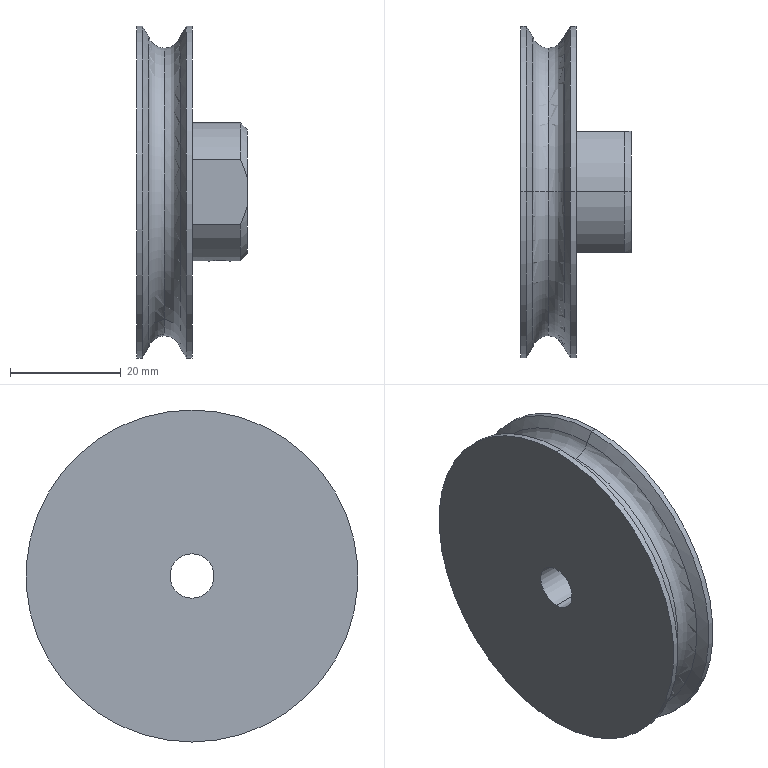Part | STEP file | 11-MBR58_3_P811 | 1 solid | 31 faces | box 20 x 60 x 60 mm | volume 27879 mm3 | cylinder 13 | cone 9 | plane 5 | torus 4 | commonest cylinder face diameters 3.242 x4 60 x4 25 x3 8 x2
STEP:
#1=CARTESIAN_POINT('',(-2.85,0.,28.064));
#2=VERTEX_POINT('',#1);
#3=CARTESIAN_POINT('',(0.,0.,26.));
#4=VERTEX_POINT('',#3);
#5=CARTESIAN_POINT('',(0.,0.,29.));
#6=DIRECTION('',(0.,-1.,0.));
#7=DIRECTION('',(0.,0.,-1.));
#8=AXIS2_PLACEMENT_3D('',#5,#6,#7);
#9=CIRCLE('',#8,3.);
#10=EDGE_CURVE('',#2,#4,#9,.T.);
#11=ORIENTED_EDGE('',*,*,#10,.T.);
#12=CARTESIAN_POINT('',(0.,0.,-26.));
#13=VERTEX_POINT('',#12);
#14=CARTESIAN_POINT('',(0.,0.,0.));
#15=DIRECTION('',(-1.,0.,0.));
#16=DIRECTION('',(0.,0.,1.));
#17=AXIS2_PLACEMENT_3D('',#14,#15,#16);
#18=CIRCLE('',#17,26.);
#19=EDGE_CURVE('',#4,#13,#18,.T.);
#20=ORIENTED_EDGE('',*,*,#19,.T.);
#21=CARTESIAN_POINT('',(-2.85,0.,-28.064));
#22=VERTEX_POINT('',#21);
#23=CARTESIAN_POINT('',(0.,0.,-29.));
#24=DIRECTION('',(0.,1.,0.));
#25=DIRECTION('',(0.,0.,1.));
#26=AXIS2_PLACEMENT_3D('',#23,#24,#25);
#27=CIRCLE('',#26,3.);
#28=EDGE_CURVE('',#22,#13,#27,.T.);
#29=ORIENTED_EDGE('',*,*,#28,.F.);
#30=CARTESIAN_POINT('',(-2.85,0.,0.));
#31=DIRECTION('',(-1.,0.,0.));
#32=DIRECTION('',(0.,0.,1.));
#33=AXIS2_PLACEMENT_3D('',#30,#31,#32);
#34=CIRCLE('',#33,28.064);
#35=EDGE_CURVE('',#2,#22,#34,.T.);
#36=ORIENTED_EDGE('',*,*,#35,.F.);
#37=EDGE_LOOP('',(#11,#20,#29,#36));
#38=FACE_OUTER_BOUND('',#37,.T.);
#39=CARTESIAN_POINT('',(0.,0.,0.));
#40=DIRECTION('',(-1.,0.,0.));
#41=DIRECTION('',(0.,0.,1.));
#42=AXIS2_PLACEMENT_3D('',#39,#40,#41);
#43=TOROIDAL_SURFACE('',#42,29.,3.);
#44=ADVANCED_FACE('',(#38),#43,.F.);
#45=ORIENTED_EDGE('',*,*,#28,.T.);
#46=CARTESIAN_POINT('',(0.,0.,0.));
#47=DIRECTION('',(-1.,0.,0.));
#48=DIRECTION('',(0.,0.,1.));
#49=AXIS2_PLACEMENT_3D('',#46,#47,#48);
#50=CIRCLE('',#49,26.);
#51=EDGE_CURVE('',#13,#4,#50,.T.);
#52=ORIENTED_EDGE('',*,*,#51,.T.);
#53=ORIENTED_EDGE('',*,*,#10,.F.);
#54=CARTESIAN_POINT('',(-2.85,0.,0.));
#55=DIRECTION('',(-1.,0.,0.));
#56=DIRECTION('',(0.,0.,1.));
#57=AXIS2_PLACEMENT_3D('',#54,#55,#56);
#58=CIRCLE('',#57,28.064);
#59=EDGE_CURVE('',#22,#2,#58,.T.);
#60=ORIENTED_EDGE('',*,*,#59,.F.);
#61=EDGE_LOOP('',(#45,#52,#53,#60));
#62=FACE_OUTER_BOUND('',#61,.T.);
#63=CARTESIAN_POINT('',(0.,0.,0.));
#64=DIRECTION('',(-1.,0.,0.));
#65=DIRECTION('',(0.,0.,1.));
#66=AXIS2_PLACEMENT_3D('',#63,#64,#65);
#67=TOROIDAL_SURFACE('',#66,29.,3.);
#68=ADVANCED_FACE('',(#62),#67,.F.);
#69=CARTESIAN_POINT('',(8.379,0.,-4.));
#70=VERTEX_POINT('',#69);
#71=CARTESIAN_POINT('',(11.621,0.,-4.));
#72=VERTEX_POINT('',#71);
#73=CARTESIAN_POINT('',(8.379,0.,-4.));
#74=CARTESIAN_POINT('',(8.379,-0.1084,-4.));
#75=CARTESIAN_POINT('',(8.39,-0.2147,-3.996));
#76=CARTESIAN_POINT('',(8.432,-0.4235,-3.979));
#77=CARTESIAN_POINT('',(8.463,-0.5271,-3.966));
#78=CARTESIAN_POINT('',(8.586,-0.821,-3.92));
#79=CARTESIAN_POINT('',(8.707,-0.9992,-3.876));
#80=CARTESIAN_POINT('',(9.002,-1.295,-3.788));
#81=CARTESIAN_POINT('',(9.181,-1.415,-3.742));
#82=CARTESIAN_POINT('',(9.473,-1.537,-3.693));
#83=CARTESIAN_POINT('',(9.576,-1.568,-3.68));
#84=CARTESIAN_POINT('',(9.786,-1.61,-3.662));
#85=CARTESIAN_POINT('',(9.892,-1.621,-3.657));
#86=CARTESIAN_POINT('',(10.106,-1.621,-3.657));
#87=CARTESIAN_POINT('',(10.215,-1.61,-3.662));
#88=CARTESIAN_POINT('',(10.424,-1.568,-3.68));
#89=CARTESIAN_POINT('',(10.526,-1.537,-3.693));
#90=CARTESIAN_POINT('',(10.723,-1.455,-3.726));
#91=CARTESIAN_POINT('',(10.816,-1.405,-3.746));
#92=CARTESIAN_POINT('',(10.99,-1.288,-3.788));
#93=CARTESIAN_POINT('',(11.073,-1.22,-3.81));
#94=CARTESIAN_POINT('',(11.221,-1.072,-3.855));
#95=CARTESIAN_POINT('',(11.287,-0.9909,-3.876));
#96=CARTESIAN_POINT('',(11.405,-0.8157,-3.917));
#97=CARTESIAN_POINT('',(11.456,-0.7213,-3.936));
#98=CARTESIAN_POINT('',(11.577,-0.429,-3.982));
#99=CARTESIAN_POINT('',(11.621,-0.2135,-4.));
#100=CARTESIAN_POINT('',(11.621,0.,-4.));
#101=B_SPLINE_CURVE_WITH_KNOTS('',3,(#73,#74,#75,#76,#77,#78,#79,#80,#81,#82,#83,#84,#85,#86,#87,#88,#89,#90,#91,#92,#93,#94,#95,#96,#97,#98,#99,#100),.UNSPECIFIED.,.F.,.F.,(4,2,2,2,2,2,2,2,2,2,2,2,2,4),(0.,0.0003202,0.0006405,0.001281,0.001921,0.002242,0.002562,0.002882,0.003202,0.003523,0.003843,0.004163,0.004483,0.005124),.UNSPECIFIED.);
#102=EDGE_CURVE('',#70,#72,#101,.T.);
#103=ORIENTED_EDGE('',*,*,#102,.T.);
#104=CARTESIAN_POINT('',(11.621,0.,-12.121));
#105=VERTEX_POINT('',#104);
#106=CARTESIAN_POINT('',(11.621,0.,-3.));
#107=DIRECTION('',(0.,0.,-1.));
#108=VECTOR('',#107,1000.);
#109=LINE('',#106,#108);
#110=EDGE_CURVE('',#72,#105,#109,.T.);
#111=ORIENTED_EDGE('',*,*,#110,.T.);
#112=CARTESIAN_POINT('',(8.379,0.,-12.121));
#113=VERTEX_POINT('',#112);
#114=CARTESIAN_POINT('',(10.,0.,-12.121));
#115=DIRECTION('',(0.,0.,-1.));
#116=DIRECTION('',(-1.,0.,0.));
#117=AXIS2_PLACEMENT_3D('',#114,#115,#116);
#118=CIRCLE('',#117,1.621);
#119=EDGE_CURVE('',#105,#113,#118,.T.);
#120=ORIENTED_EDGE('',*,*,#119,.T.);
#121=CARTESIAN_POINT('',(8.379,0.,-3.));
#122=DIRECTION('',(0.,0.,-1.));
#123=VECTOR('',#122,1000.);
#124=LINE('',#121,#123);
#125=EDGE_CURVE('',#70,#113,#124,.T.);
#126=ORIENTED_EDGE('',*,*,#125,.F.);
#127=EDGE_LOOP('',(#103,#111,#120,#126));
#128=FACE_OUTER_BOUND('',#127,.T.);
#129=CARTESIAN_POINT('',(10.,0.,-3.));
#130=DIRECTION('',(0.,0.,-1.));
#131=DIRECTION('',(-1.,0.,0.));
#132=AXIS2_PLACEMENT_3D('',#129,#130,#131);
#133=CYLINDRICAL_SURFACE('',#132,1.621);
#134=ADVANCED_FACE('',(#128),#133,.F.);
#135=ORIENTED_EDGE('',*,*,#119,.F.);
#136=CARTESIAN_POINT('',(12.,0.,-12.5));
#137=VERTEX_POINT('',#136);
#138=CARTESIAN_POINT('',(11.621,0.,-12.121));
#139=DIRECTION('',(0.7071,0.,-0.7071));
#140=VECTOR('',#139,1000.);
#141=LINE('',#138,#140);
#142=EDGE_CURVE('',#105,#137,#141,.T.);
#143=ORIENTED_EDGE('',*,*,#142,.T.);
#144=CARTESIAN_POINT('',(8.,0.,-12.5));
#145=VERTEX_POINT('',#144);
#146=CARTESIAN_POINT('',(12.,0.,-12.5));
#147=CARTESIAN_POINT('',(12.,-0.2539,-12.5));
#148=CARTESIAN_POINT('',(11.943,-0.5065,-12.492));
#149=CARTESIAN_POINT('',(11.783,-0.8509,-12.472));
#150=CARTESIAN_POINT('',(11.718,-0.9588,-12.464));
#151=CARTESIAN_POINT('',(11.567,-1.162,-12.446));
#152=CARTESIAN_POINT('',(11.48,-1.256,-12.437));
#153=CARTESIAN_POINT('',(11.199,-1.507,-12.41));
#154=CARTESIAN_POINT('',(10.978,-1.64,-12.392));
#155=CARTESIAN_POINT('',(10.624,-1.772,-12.374));
#156=CARTESIAN_POINT('',(10.5,-1.805,-12.369));
#157=CARTESIAN_POINT('',(10.251,-1.85,-12.362));
#158=CARTESIAN_POINT('',(10.126,-1.861,-12.361));
#159=CARTESIAN_POINT('',(9.873,-1.861,-12.361));
#160=CARTESIAN_POINT('',(9.745,-1.849,-12.362));
#161=CARTESIAN_POINT('',(9.497,-1.805,-12.369));
#162=CARTESIAN_POINT('',(9.376,-1.771,-12.374));
#163=CARTESIAN_POINT('',(9.139,-1.683,-12.386));
#164=CARTESIAN_POINT('',(9.024,-1.628,-12.394));
#165=CARTESIAN_POINT('',(8.808,-1.498,-12.41));
#166=CARTESIAN_POINT('',(8.706,-1.423,-12.419));
#167=CARTESIAN_POINT('',(8.517,-1.253,-12.437));
#168=CARTESIAN_POINT('',(8.432,-1.16,-12.446));
#169=CARTESIAN_POINT('',(8.281,-0.9576,-12.464));
#170=CARTESIAN_POINT('',(8.215,-0.8474,-12.472));
#171=CARTESIAN_POINT('',(8.057,-0.5052,-12.492));
#172=CARTESIAN_POINT('',(8.,-0.2516,-12.5));
#173=CARTESIAN_POINT('',(8.,0.,-12.5));
#174=B_SPLINE_CURVE_WITH_KNOTS('',3,(#146,#147,#148,#149,#150,#151,#152,#153,#154,#155,#156,#157,#158,#159,#160,#161,#162,#163,#164,#165,#166,#167,#168,#169,#170,#171,#172,#173),.UNSPECIFIED.,.F.,.F.,(4,2,2,2,2,2,2,2,2,2,2,2,2,4),(0.007606,0.008363,0.008741,0.00912,0.009877,0.01026,0.01063,0.01101,0.01139,0.01177,0.01215,0.01253,0.0129,0.01366),.UNSPECIFIED.);
#175=EDGE_CURVE('',#137,#145,#174,.T.);
#176=ORIENTED_EDGE('',*,*,#175,.T.);
#177=CARTESIAN_POINT('',(8.379,0.,-12.121));
#178=DIRECTION('',(-0.7071,0.,-0.7071));
#179=VECTOR('',#178,1000.);
#180=LINE('',#177,#179);
#181=EDGE_CURVE('',#113,#145,#180,.T.);
#182=ORIENTED_EDGE('',*,*,#181,.F.);
#183=EDGE_LOOP('',(#135,#143,#176,#182));
#184=FACE_OUTER_BOUND('',#183,.T.);
#185=CARTESIAN_POINT('',(10.,0.,-12.121));
#186=DIRECTION('',(0.,0.,-1.));
#187=DIRECTION('',(-1.,0.,0.));
#188=AXIS2_PLACEMENT_3D('',#185,#186,#187);
#189=CONICAL_SURFACE('',#188,1.621,0.7854);
#190=ADVANCED_FACE('',(#184),#189,.F.);
#191=CARTESIAN_POINT('',(10.,3.657,1.621));
#192=VERTEX_POINT('',#191);
#193=CARTESIAN_POINT('',(10.,3.657,-1.621));
#194=VERTEX_POINT('',#193);
#195=CARTESIAN_POINT('',(10.,3.657,1.621));
#196=CARTESIAN_POINT('',(9.892,3.657,1.621));
#197=CARTESIAN_POINT('',(9.785,3.662,1.61));
#198=CARTESIAN_POINT('',(9.577,3.68,1.568));
#199=CARTESIAN_POINT('',(9.473,3.693,1.537));
#200=CARTESIAN_POINT('',(9.18,3.743,1.414));
#201=CARTESIAN_POINT('',(9.002,3.788,1.294));
#202=CARTESIAN_POINT('',(8.706,3.876,0.9983));
#203=CARTESIAN_POINT('',(8.586,3.92,0.8195));
#204=CARTESIAN_POINT('',(8.464,3.966,0.5273));
#205=CARTESIAN_POINT('',(8.432,3.979,0.4239));
#206=CARTESIAN_POINT('',(8.39,3.996,0.214));
#207=CARTESIAN_POINT('',(8.379,4.,0.108));
#208=CARTESIAN_POINT('',(8.379,4.,-0.1063));
#209=CARTESIAN_POINT('',(8.39,3.996,-0.2149));
#210=CARTESIAN_POINT('',(8.432,3.979,-0.424));
#211=CARTESIAN_POINT('',(8.463,3.967,-0.5259));
#212=CARTESIAN_POINT('',(8.545,3.935,-0.7235));
#213=CARTESIAN_POINT('',(8.596,3.917,-0.8164));
#214=CARTESIAN_POINT('',(8.713,3.876,-0.9909));
#215=CARTESIAN_POINT('',(8.781,3.854,-1.073));
#216=CARTESIAN_POINT('',(8.929,3.81,-1.221));
#217=CARTESIAN_POINT('',(9.01,3.788,-1.288));
#218=CARTESIAN_POINT('',(9.185,3.746,-1.405));
#219=CARTESIAN_POINT('',(9.279,3.726,-1.456));
#220=CARTESIAN_POINT('',(9.571,3.677,-1.577));
#221=CARTESIAN_POINT('',(9.787,3.657,-1.621));
#222=CARTESIAN_POINT('',(10.,3.657,-1.621));
#223=B_SPLINE_CURVE_WITH_KNOTS('',3,(#195,#196,#197,#198,#199,#200,#201,#202,#203,#204,#205,#206,#207,#208,#209,#210,#211,#212,#213,#214,#215,#216,#217,#218,#219,#220,#221,#222),.UNSPECIFIED.,.F.,.F.,(4,2,2,2,2,2,2,2,2,2,2,2,2,4),(0.,0.0003202,0.0006404,0.001281,0.001921,0.002242,0.002562,0.002882,0.003202,0.003522,0.003843,0.004163,0.004483,0.005123),.UNSPECIFIED.);
#224=EDGE_CURVE('',#192,#194,#223,.T.);
#225=ORIENTED_EDGE('',*,*,#224,.T.);
#226=CARTESIAN_POINT('',(10.,11.,-1.621));
#227=VERTEX_POINT('',#226);
#228=CARTESIAN_POINT('',(10.,3.,-1.621));
#229=DIRECTION('',(0.,1.,0.));
#230=VECTOR('',#229,1000.);
#231=LINE('',#228,#230);
#232=EDGE_CURVE('',#194,#227,#231,.T.);
#233=ORIENTED_EDGE('',*,*,#232,.T.);
#234=CARTESIAN_POINT('',(10.,11.,1.621));
#235=VERTEX_POINT('',#234);
#236=CARTESIAN_POINT('',(10.,11.,0.));
#237=DIRECTION('',(0.,-1.,0.));
#238=DIRECTION('',(0.,0.,-1.));
#239=AXIS2_PLACEMENT_3D('',#236,#237,#238);
#240=CIRCLE('',#239,1.621);
#241=EDGE_CURVE('',#235,#227,#240,.T.);
#242=ORIENTED_EDGE('',*,*,#241,.F.);
#243=CARTESIAN_POINT('',(10.,3.,1.621));
#244=DIRECTION('',(0.,1.,0.));
#245=VECTOR('',#244,1000.);
#246=LINE('',#243,#245);
#247=EDGE_CURVE('',#192,#235,#246,.T.);
#248=ORIENTED_EDGE('',*,*,#247,.F.);
#249=EDGE_LOOP('',(#225,#233,#242,#248));
#250=FACE_OUTER_BOUND('',#249,.T.);
#251=CARTESIAN_POINT('',(10.,3.,0.));
#252=DIRECTION('',(0.,1.,0.));
#253=DIRECTION('',(0.,0.,1.));
#254=AXIS2_PLACEMENT_3D('',#251,#252,#253);
#255=CYLINDRICAL_SURFACE('',#254,1.621);
#256=ADVANCED_FACE('',(#250),#255,.F.);
#257=CARTESIAN_POINT('',(5.,0.,30.));
#258=VERTEX_POINT('',#257);
#259=CARTESIAN_POINT('',(5.,0.,-30.));
#260=VERTEX_POINT('',#259);
#261=CARTESIAN_POINT('',(5.,0.,0.));
#262=DIRECTION('',(-1.,0.,0.));
#263=DIRECTION('',(0.,0.,1.));
#264=AXIS2_PLACEMENT_3D('',#261,#262,#263);
#265=CIRCLE('',#264,30.);
#266=EDGE_CURVE('',#258,#260,#265,.T.);
#267=ORIENTED_EDGE('',*,*,#266,.T.);
#268=CARTESIAN_POINT('',(3.968,0.,-30.));
#269=VERTEX_POINT('',#268);
#270=CARTESIAN_POINT('',(15.,0.,-30.));
#271=DIRECTION('',(-1.,0.,0.));
#272=VECTOR('',#271,1000.);
#273=LINE('',#270,#272);
#274=EDGE_CURVE('',#260,#269,#273,.T.);
#275=ORIENTED_EDGE('',*,*,#274,.T.);
#276=CARTESIAN_POINT('',(3.968,0.,30.));
#277=VERTEX_POINT('',#276);
#278=CARTESIAN_POINT('',(3.968,0.,0.));
#279=DIRECTION('',(-1.,0.,0.));
#280=DIRECTION('',(0.,0.,1.));
#281=AXIS2_PLACEMENT_3D('',#278,#279,#280);
#282=CIRCLE('',#281,30.);
#283=EDGE_CURVE('',#277,#269,#282,.T.);
#284=ORIENTED_EDGE('',*,*,#283,.F.);
#285=CARTESIAN_POINT('',(15.,0.,30.));
#286=DIRECTION('',(-1.,0.,0.));
#287=VECTOR('',#286,1000.);
#288=LINE('',#285,#287);
#289=EDGE_CURVE('',#258,#277,#288,.T.);
#290=ORIENTED_EDGE('',*,*,#289,.F.);
#291=EDGE_LOOP('',(#267,#275,#284,#290));
#292=FACE_OUTER_BOUND('',#291,.T.);
#293=CARTESIAN_POINT('',(15.,0.,0.));
#294=DIRECTION('',(-1.,0.,0.));
#295=DIRECTION('',(0.,0.,1.));
#296=AXIS2_PLACEMENT_3D('',#293,#294,#295);
#297=CYLINDRICAL_SURFACE('',#296,30.);
#298=ADVANCED_FACE('',(#292),#297,.T.);
#299=CARTESIAN_POINT('',(2.85,0.,28.064));
#300=VERTEX_POINT('',#299);
#301=CARTESIAN_POINT('',(2.85,0.,-28.064));
#302=VERTEX_POINT('',#301);
#303=CARTESIAN_POINT('',(2.85,0.,0.));
#304=DIRECTION('',(-1.,0.,0.));
#305=DIRECTION('',(0.,0.,1.));
#306=AXIS2_PLACEMENT_3D('',#303,#304,#305);
#307=CIRCLE('',#306,28.064);
#308=EDGE_CURVE('',#300,#302,#307,.T.);
#309=ORIENTED_EDGE('',*,*,#308,.F.);
#310=CARTESIAN_POINT('',(3.968,0.,30.));
#311=DIRECTION('',(0.5,0.,0.866));
#312=VECTOR('',#311,1000.);
#313=LINE('',#310,#312);
#314=EDGE_CURVE('',#300,#277,#313,.T.);
#315=ORIENTED_EDGE('',*,*,#314,.T.);
#316=ORIENTED_EDGE('',*,*,#283,.T.);
#317=CARTESIAN_POINT('',(3.968,0.,-30.));
#318=DIRECTION('',(0.5,0.,-0.866));
#319=VECTOR('',#318,1000.);
#320=LINE('',#317,#319);
#321=EDGE_CURVE('',#302,#269,#320,.T.);
#322=ORIENTED_EDGE('',*,*,#321,.F.);
#323=EDGE_LOOP('',(#309,#315,#316,#322));
#324=FACE_OUTER_BOUND('',#323,.T.);
#325=CARTESIAN_POINT('',(3.968,0.,0.));
#326=DIRECTION('',(1.,0.,0.));
#327=DIRECTION('',(0.,0.,-1.));
#328=AXIS2_PLACEMENT_3D('',#325,#326,#327);
#329=CONICAL_SURFACE('',#328,30.,1.047);
#330=ADVANCED_FACE('',(#324),#329,.T.);
#331=ORIENTED_EDGE('',*,*,#51,.F.);
#332=CARTESIAN_POINT('',(0.,0.,-29.));
#333=DIRECTION('',(0.,1.,0.));
#334=DIRECTION('',(0.,0.,1.));
#335=AXIS2_PLACEMENT_3D('',#332,#333,#334);
#336=CIRCLE('',#335,3.);
#337=EDGE_CURVE('',#13,#302,#336,.T.);
#338=ORIENTED_EDGE('',*,*,#337,.T.);
#339=CARTESIAN_POINT('',(2.85,0.,0.));
#340=DIRECTION('',(-1.,0.,0.));
#341=DIRECTION('',(0.,0.,1.));
#342=AXIS2_PLACEMENT_3D('',#339,#340,#341);
#343=CIRCLE('',#342,28.064);
#344=EDGE_CURVE('',#302,#300,#343,.T.);
#345=ORIENTED_EDGE('',*,*,#344,.T.);
#346=CARTESIAN_POINT('',(0.,0.,29.));
#347=DIRECTION('',(0.,-1.,0.));
#348=DIRECTION('',(0.,0.,-1.));
#349=AXIS2_PLACEMENT_3D('',#346,#347,#348);
#350=CIRCLE('',#349,3.);
#351=EDGE_CURVE('',#4,#300,#350,.T.);
#352=ORIENTED_EDGE('',*,*,#351,.F.);
#353=EDGE_LOOP('',(#331,#338,#345,#352));
#354=FACE_OUTER_BOUND('',#353,.T.);
#355=CARTESIAN_POINT('',(0.,0.,0.));
#356=DIRECTION('',(-1.,0.,0.));
#357=DIRECTION('',(0.,0.,1.));
#358=AXIS2_PLACEMENT_3D('',#355,#356,#357);
#359=TOROIDAL_SURFACE('',#358,29.,3.);
#360=ADVANCED_FACE('',(#354),#359,.F.);
#361=ORIENTED_EDGE('',*,*,#35,.T.);
#362=CARTESIAN_POINT('',(-3.968,0.,-30.));
#363=VERTEX_POINT('',#362);
#364=CARTESIAN_POINT('',(-2.85,0.,-28.064));
#365=DIRECTION('',(-0.5,0.,-0.866));
#366=VECTOR('',#365,1000.);
#367=LINE('',#364,#366);
#368=EDGE_CURVE('',#22,#363,#367,.T.);
#369=ORIENTED_EDGE('',*,*,#368,.T.);
#370=CARTESIAN_POINT('',(-3.968,0.,30.));
#371=VERTEX_POINT('',#370);
#372=CARTESIAN_POINT('',(-3.968,0.,0.));
#373=DIRECTION('',(-1.,0.,0.));
#374=DIRECTION('',(0.,0.,1.));
#375=AXIS2_PLACEMENT_3D('',#372,#373,#374);
#376=CIRCLE('',#375,30.);
#377=EDGE_CURVE('',#371,#363,#376,.T.);
#378=ORIENTED_EDGE('',*,*,#377,.F.);
#379=CARTESIAN_POINT('',(-2.85,0.,28.064));
#380=DIRECTION('',(-0.5,0.,0.866));
#381=VECTOR('',#380,1000.);
#382=LINE('',#379,#381);
#383=EDGE_CURVE('',#2,#371,#382,.T.);
#384=ORIENTED_EDGE('',*,*,#383,.F.);
#385=EDGE_LOOP('',(#361,#369,#378,#384));
#386=FACE_OUTER_BOUND('',#385,.T.);
#387=CARTESIAN_POINT('',(-2.85,0.,0.));
#388=DIRECTION('',(-1.,0.,0.));
#389=DIRECTION('',(0.,0.,1.));
#390=AXIS2_PLACEMENT_3D('',#387,#388,#389);
#391=CONICAL_SURFACE('',#390,28.064,1.047);
#392=ADVANCED_FACE('',(#386),#391,.T.);
#393=ORIENTED_EDGE('',*,*,#377,.T.);
#394=CARTESIAN_POINT('',(-5.,0.,-30.));
#395=VERTEX_POINT('',#394);
#396=CARTESIAN_POINT('',(15.,0.,-30.));
#397=DIRECTION('',(-1.,0.,0.));
#398=VECTOR('',#397,1000.);
#399=LINE('',#396,#398);
#400=EDGE_CURVE('',#363,#395,#399,.T.);
#401=ORIENTED_EDGE('',*,*,#400,.T.);
#402=CARTESIAN_POINT('',(-5.,0.,30.));
#403=VERTEX_POINT('',#402);
#404=CARTESIAN_POINT('',(-5.,0.,0.));
#405=DIRECTION('',(-1.,0.,0.));
#406=DIRECTION('',(0.,0.,1.));
#407=AXIS2_PLACEMENT_3D('',#404,#405,#406);
#408=CIRCLE('',#407,30.);
#409=EDGE_CURVE('',#403,#395,#408,.T.);
#410=ORIENTED_EDGE('',*,*,#409,.F.);
#411=CARTESIAN_POINT('',(15.,0.,30.));
#412=DIRECTION('',(-1.,0.,0.));
#413=VECTOR('',#412,1000.);
#414=LINE('',#411,#413);
#415=EDGE_CURVE('',#371,#403,#414,.T.);
#416=ORIENTED_EDGE('',*,*,#415,.F.);
#417=EDGE_LOOP('',(#393,#401,#410,#416));
#418=FACE_OUTER_BOUND('',#417,.T.);
#419=CARTESIAN_POINT('',(15.,0.,0.));
#420=DIRECTION('',(-1.,0.,0.));
#421=DIRECTION('',(0.,0.,1.));
#422=AXIS2_PLACEMENT_3D('',#419,#420,#421);
#423=CYLINDRICAL_SURFACE('',#422,30.);
#424=ADVANCED_FACE('',(#418),#423,.T.);
#425=CARTESIAN_POINT('',(15.,0.,-4.));
#426=VERTEX_POINT('',#425);
#427=CARTESIAN_POINT('',(15.,0.,4.));
#428=VERTEX_POINT('',#427);
#429=CARTESIAN_POINT('',(15.,0.,0.));
#430=DIRECTION('',(-1.,0.,0.));
#431=DIRECTION('',(0.,0.,1.));
#432=AXIS2_PLACEMENT_3D('',#429,#430,#431);
#433=CIRCLE('',#432,4.);
#434=EDGE_CURVE('',#426,#428,#433,.T.);
#435=ORIENTED_EDGE('',*,*,#434,.F.);
#436=CARTESIAN_POINT('',(15.,0.,-4.));
#437=DIRECTION('',(-1.,0.,0.));
#438=VECTOR('',#437,1000.);
#439=LINE('',#436,#438);
#440=EDGE_CURVE('',#426,#72,#439,.T.);
#441=ORIENTED_EDGE('',*,*,#440,.T.);
#442=ORIENTED_EDGE('',*,*,#102,.F.);
#443=CARTESIAN_POINT('',(-5.,0.,-4.));
#444=VERTEX_POINT('',#443);
#445=CARTESIAN_POINT('',(15.,0.,-4.));
#446=DIRECTION('',(-1.,0.,0.));
#447=VECTOR('',#446,1000.);
#448=LINE('',#445,#447);
#449=EDGE_CURVE('',#70,#444,#448,.T.);
#450=ORIENTED_EDGE('',*,*,#449,.T.);
#451=CARTESIAN_POINT('',(-5.,0.,4.));
#452=VERTEX_POINT('',#451);
#453=CARTESIAN_POINT('',(-5.,0.,0.));
#454=DIRECTION('',(-1.,0.,0.));
#455=DIRECTION('',(0.,0.,1.));
#456=AXIS2_PLACEMENT_3D('',#453,#454,#455);
#457=CIRCLE('',#456,4.);
#458=EDGE_CURVE('',#444,#452,#457,.T.);
#459=ORIENTED_EDGE('',*,*,#458,.T.);
#460=CARTESIAN_POINT('',(15.,0.,4.));
#461=DIRECTION('',(-1.,0.,0.));
#462=VECTOR('',#461,1000.);
#463=LINE('',#460,#462);
#464=EDGE_CURVE('',#428,#452,#463,.T.);
#465=ORIENTED_EDGE('',*,*,#464,.F.);
#466=EDGE_LOOP('',(#435,#441,#442,#450,#459,#465));
#467=FACE_OUTER_BOUND('',#466,.T.);
#468=CARTESIAN_POINT('',(15.,0.,0.));
#469=DIRECTION('',(-1.,0.,0.));
#470=DIRECTION('',(0.,0.,1.));
#471=AXIS2_PLACEMENT_3D('',#468,#469,#470);
#472=CYLINDRICAL_SURFACE('',#471,4.);
#473=ADVANCED_FACE('',(#467),#472,.F.);
#474=CARTESIAN_POINT('',(13.75,-11.,5.937));
#475=VERTEX_POINT('',#474);
#476=CARTESIAN_POINT('',(13.75,0.,12.5));
#477=VERTEX_POINT('',#476);
#478=CARTESIAN_POINT('',(13.75,0.,0.));
#479=DIRECTION('',(-1.,0.,0.));
#480=DIRECTION('',(0.,0.,1.));
#481=AXIS2_PLACEMENT_3D('',#478,#479,#480);
#482=CIRCLE('',#481,12.5);
#483=EDGE_CURVE('',#475,#477,#482,.T.);
#484=ORIENTED_EDGE('',*,*,#483,.T.);
#485=CARTESIAN_POINT('',(5.,0.,12.5));
#486=VERTEX_POINT('',#485);
#487=CARTESIAN_POINT('',(15.,0.,12.5));
#488=DIRECTION('',(-1.,0.,0.));
#489=VECTOR('',#488,1000.);
#490=LINE('',#487,#489);
#491=EDGE_CURVE('',#477,#486,#490,.T.);
#492=ORIENTED_EDGE('',*,*,#491,.T.);
#493=CARTESIAN_POINT('',(5.,-11.,5.937));
#494=VERTEX_POINT('',#493);
#495=CARTESIAN_POINT('',(5.,0.,0.));
#496=DIRECTION('',(-1.,0.,0.));
#497=DIRECTION('',(0.,0.,1.));
#498=AXIS2_PLACEMENT_3D('',#495,#496,#497);
#499=CIRCLE('',#498,12.5);
#500=EDGE_CURVE('',#494,#486,#499,.T.);
#501=ORIENTED_EDGE('',*,*,#500,.F.);
#502=CARTESIAN_POINT('',(-6.969,-11.,5.937));
#503=DIRECTION('',(1.,0.,0.));
#504=VECTOR('',#503,1000.);
#505=LINE('',#502,#504);
#506=EDGE_CURVE('',#494,#475,#505,.T.);
#507=ORIENTED_EDGE('',*,*,#506,.T.);
#508=EDGE_LOOP('',(#484,#492,#501,#507));
#509=FACE_OUTER_BOUND('',#508,.T.);
#510=CARTESIAN_POINT('',(15.,0.,0.));
#511=DIRECTION('',(-1.,0.,0.));
#512=DIRECTION('',(0.,0.,1.));
#513=AXIS2_PLACEMENT_3D('',#510,#511,#512);
#514=CYLINDRICAL_SURFACE('',#513,12.5);
#515=ADVANCED_FACE('',(#509),#514,.T.);
#516=CARTESIAN_POINT('',(15.,-11.,2.358));
#517=VERTEX_POINT('',#516);
#518=CARTESIAN_POINT('',(15.,0.,11.25));
#519=VERTEX_POINT('',#518);
#520=CARTESIAN_POINT('',(15.,0.,0.));
#521=DIRECTION('',(-1.,0.,0.));
#522=DIRECTION('',(0.,0.,1.));
#523=AXIS2_PLACEMENT_3D('',#520,#521,#522);
#524=CIRCLE('',#523,11.25);
#525=EDGE_CURVE('',#517,#519,#524,.T.);
#526=ORIENTED_EDGE('',*,*,#525,.T.);
#527=CARTESIAN_POINT('',(15.,0.,11.25));
#528=DIRECTION('',(-0.7071,0.,0.7071));
#529=VECTOR('',#528,1000.);
#530=LINE('',#527,#529);
#531=EDGE_CURVE('',#519,#477,#530,.T.);
#532=ORIENTED_EDGE('',*,*,#531,.T.);
#533=ORIENTED_EDGE('',*,*,#483,.F.);
#534=CARTESIAN_POINT('',(13.75,-11.,5.937));
#535=CARTESIAN_POINT('',(13.885,-11.,5.652));
#536=CARTESIAN_POINT('',(14.015,-11.,5.364));
#537=CARTESIAN_POINT('',(14.26,-11.,4.778));
#538=CARTESIAN_POINT('',(14.376,-11.,4.48));
#539=CARTESIAN_POINT('',(14.696,-11.,3.58));
#540=CARTESIAN_POINT('',(14.871,-11.,2.974));
#541=CARTESIAN_POINT('',(15.,-11.,2.358));
#542=B_SPLINE_CURVE_WITH_KNOTS('',3,(#534,#535,#536,#537,#538,#539,#540,#541),.UNSPECIFIED.,.F.,.F.,(4,2,2,4),(0.008515,0.009456,0.0104,0.01228),.UNSPECIFIED.);
#543=EDGE_CURVE('',#475,#517,#542,.T.);
#544=ORIENTED_EDGE('',*,*,#543,.T.);
#545=EDGE_LOOP('',(#526,#532,#533,#544));
#546=FACE_OUTER_BOUND('',#545,.T.);
#547=CARTESIAN_POINT('',(15.,0.,0.));
#548=DIRECTION('',(-1.,0.,0.));
#549=DIRECTION('',(0.,0.,1.));
#550=AXIS2_PLACEMENT_3D('',#547,#548,#549);
#551=CONICAL_SURFACE('',#550,11.25,0.7854);
#552=ADVANCED_FACE('',(#546),#551,.T.);
#553=CARTESIAN_POINT('',(8.,0.,-12.5));
#554=CARTESIAN_POINT('',(8.,0.1259,-12.5));
#555=CARTESIAN_POINT('',(8.014,0.2537,-12.498));
#556=CARTESIAN_POINT('',(8.069,0.501,-12.491));
#557=CARTESIAN_POINT('',(8.11,0.6202,-12.485));
#558=CARTESIAN_POINT('',(8.27,0.9652,-12.465));
#559=CARTESIAN_POINT('',(8.425,1.171,-12.446));
#560=CARTESIAN_POINT('',(8.708,1.425,-12.419));
#561=CARTESIAN_POINT('',(8.81,1.499,-12.41));
#562=CARTESIAN_POINT('',(9.026,1.629,-12.394));
#563=CARTESIAN_POINT('',(9.142,1.684,-12.386));
#564=CARTESIAN_POINT('',(9.496,1.816,-12.368));
#565=CARTESIAN_POINT('',(9.751,1.861,-12.361));
#566=CARTESIAN_POINT('',(10.255,1.86,-12.361));
#567=CARTESIAN_POINT('',(10.509,1.815,-12.368));
#568=CARTESIAN_POINT('',(10.98,1.638,-12.392));
#569=CARTESIAN_POINT('',(11.202,1.505,-12.41));
#570=CARTESIAN_POINT('',(11.482,1.254,-12.437));
#571=CARTESIAN_POINT('',(11.568,1.16,-12.446));
#572=CARTESIAN_POINT('',(11.72,0.9568,-12.464));
#573=CARTESIAN_POINT('',(11.784,0.849,-12.472));
#574=CARTESIAN_POINT('',(11.89,0.6208,-12.485));
#575=CARTESIAN_POINT('',(11.931,0.4987,-12.491));
#576=CARTESIAN_POINT('',(11.986,0.2522,-12.498));
#577=CARTESIAN_POINT('',(12.,0.1271,-12.5));
#578=CARTESIAN_POINT('',(12.,0.,-12.5));
#579=B_SPLINE_CURVE_WITH_KNOTS('',3,(#553,#554,#555,#556,#557,#558,#559,#560,#561,#562,#563,#564,#565,#566,#567,#568,#569,#570,#571,#572,#573,#574,#575,#576,#577,#578),.UNSPECIFIED.,.F.,.F.,(4,2,2,2,2,2,2,2,2,2,2,2,4),(0.001544,0.001923,0.002301,0.003059,0.003438,0.003817,0.004575,0.005332,0.00609,0.006469,0.006848,0.007227,0.007606),.UNSPECIFIED.);
#580=EDGE_CURVE('',#145,#137,#579,.T.);
#581=ORIENTED_EDGE('',*,*,#580,.F.);
#582=ORIENTED_EDGE('',*,*,#175,.F.);
#583=EDGE_LOOP('',(#581,#582));
#584=FACE_BOUND('',#583,.T.);
#585=CARTESIAN_POINT('',(13.75,11.,-5.937));
#586=VERTEX_POINT('',#585);
#587=CARTESIAN_POINT('',(13.75,-11.,-5.937));
#588=VERTEX_POINT('',#587);
#589=CARTESIAN_POINT('',(13.75,0.,0.));
#590=DIRECTION('',(-1.,0.,0.));
#591=DIRECTION('',(0.,0.,1.));
#592=AXIS2_PLACEMENT_3D('',#589,#590,#591);
#593=CIRCLE('',#592,12.5);
#594=EDGE_CURVE('',#586,#588,#593,.T.);
#595=ORIENTED_EDGE('',*,*,#594,.T.);
#596=CARTESIAN_POINT('',(5.,-11.,-5.937));
#597=VERTEX_POINT('',#596);
#598=CARTESIAN_POINT('',(-6.969,-11.,-5.937));
#599=DIRECTION('',(1.,0.,0.));
#600=VECTOR('',#599,1000.);
#601=LINE('',#598,#600);
#602=EDGE_CURVE('',#597,#588,#601,.T.);
#603=ORIENTED_EDGE('',*,*,#602,.F.);
#604=CARTESIAN_POINT('',(5.,11.,-5.937));
#605=VERTEX_POINT('',#604);
#606=CARTESIAN_POINT('',(5.,0.,0.));
#607=DIRECTION('',(-1.,0.,0.));
#608=DIRECTION('',(0.,0.,1.));
#609=AXIS2_PLACEMENT_3D('',#606,#607,#608);
#610=CIRCLE('',#609,12.5);
#611=EDGE_CURVE('',#605,#597,#610,.T.);
#612=ORIENTED_EDGE('',*,*,#611,.F.);
#613=CARTESIAN_POINT('',(-6.969,11.,-5.937));
#614=DIRECTION('',(1.,0.,0.));
#615=VECTOR('',#614,1000.);
#616=LINE('',#613,#615);
#617=EDGE_CURVE('',#605,#586,#616,.T.);
#618=ORIENTED_EDGE('',*,*,#617,.T.);
#619=EDGE_LOOP('',(#595,#603,#612,#618));
#620=FACE_OUTER_BOUND('',#619,.T.);
#621=CARTESIAN_POINT('',(15.,0.,0.));
#622=DIRECTION('',(-1.,0.,0.));
#623=DIRECTION('',(0.,0.,1.));
#624=AXIS2_PLACEMENT_3D('',#621,#622,#623);
#625=CYLINDRICAL_SURFACE('',#624,12.5);
#626=ADVANCED_FACE('',(#584,#620),#625,.T.);
#627=ORIENTED_EDGE('',*,*,#531,.F.);
#628=CARTESIAN_POINT('',(15.,11.,2.358));
#629=VERTEX_POINT('',#628);
#630=CARTESIAN_POINT('',(15.,0.,0.));
#631=DIRECTION('',(-1.,0.,0.));
#632=DIRECTION('',(0.,0.,1.));
#633=AXIS2_PLACEMENT_3D('',#630,#631,#632);
#634=CIRCLE('',#633,11.25);
#635=EDGE_CURVE('',#519,#629,#634,.T.);
#636=ORIENTED_EDGE('',*,*,#635,.T.);
#637=CARTESIAN_POINT('',(13.75,11.,5.937));
#638=VERTEX_POINT('',#637);
#639=CARTESIAN_POINT('',(15.,11.,2.358));
#640=CARTESIAN_POINT('',(14.871,11.,2.975));
#641=CARTESIAN_POINT('',(14.696,11.,3.58));
#642=CARTESIAN_POINT('',(14.272,11.,4.774));
#643=CARTESIAN_POINT('',(14.022,11.,5.364));
#644=CARTESIAN_POINT('',(13.75,11.,5.937));
#645=B_SPLINE_CURVE_WITH_KNOTS('',3,(#639,#640,#641,#642,#643,#644),.UNSPECIFIED.,.F.,.F.,(4,2,4),(0.017,0.01888,0.02076),.UNSPECIFIED.);
#646=EDGE_CURVE('',#629,#638,#645,.T.);
#647=ORIENTED_EDGE('',*,*,#646,.T.);
#648=CARTESIAN_POINT('',(13.75,0.,0.));
#649=DIRECTION('',(-1.,0.,0.));
#650=DIRECTION('',(0.,0.,1.));
#651=AXIS2_PLACEMENT_3D('',#648,#649,#650);
#652=CIRCLE('',#651,12.5);
#653=EDGE_CURVE('',#477,#638,#652,.T.);
#654=ORIENTED_EDGE('',*,*,#653,.F.);
#655=EDGE_LOOP('',(#627,#636,#647,#654));
#656=FACE_OUTER_BOUND('',#655,.T.);
#657=CARTESIAN_POINT('',(15.,0.,0.));
#658=DIRECTION('',(-1.,0.,0.));
#659=DIRECTION('',(0.,0.,1.));
#660=AXIS2_PLACEMENT_3D('',#657,#658,#659);
#661=CONICAL_SURFACE('',#660,11.25,0.7854);
#662=ADVANCED_FACE('',(#656),#661,.T.);
#663=ORIENTED_EDGE('',*,*,#491,.F.);
#664=ORIENTED_EDGE('',*,*,#653,.T.);
#665=CARTESIAN_POINT('',(5.,11.,5.937));
#666=VERTEX_POINT('',#665);
#667=CARTESIAN_POINT('',(-6.969,11.,5.937));
#668=DIRECTION('',(1.,0.,0.));
#669=VECTOR('',#668,1000.);
#670=LINE('',#667,#669);
#671=EDGE_CURVE('',#666,#638,#670,.T.);
#672=ORIENTED_EDGE('',*,*,#671,.F.);
#673=CARTESIAN_POINT('',(5.,0.,0.));
#674=DIRECTION('',(-1.,0.,0.));
#675=DIRECTION('',(0.,0.,1.));
#676=AXIS2_PLACEMENT_3D('',#673,#674,#675);
#677=CIRCLE('',#676,12.5);
#678=EDGE_CURVE('',#486,#666,#677,.T.);
#679=ORIENTED_EDGE('',*,*,#678,.F.);
#680=EDGE_LOOP('',(#663,#664,#672,#679));
#681=FACE_OUTER_BOUND('',#680,.T.);
#682=CARTESIAN_POINT('',(15.,0.,0.));
#683=DIRECTION('',(-1.,0.,0.));
#684=DIRECTION('',(0.,0.,1.));
#685=AXIS2_PLACEMENT_3D('',#682,#683,#684);
#686=CYLINDRICAL_SURFACE('',#685,12.5);
#687=ADVANCED_FACE('',(#681),#686,.T.);
#688=ORIENTED_EDGE('',*,*,#440,.F.);
#689=CARTESIAN_POINT('',(15.,0.,0.));
#690=DIRECTION('',(-1.,0.,0.));
#691=DIRECTION('',(0.,0.,1.));
#692=AXIS2_PLACEMENT_3D('',#689,#690,#691);
#693=CIRCLE('',#692,4.);
#694=EDGE_CURVE('',#428,#426,#693,.T.);
#695=ORIENTED_EDGE('',*,*,#694,.F.);
#696=ORIENTED_EDGE('',*,*,#464,.T.);
#697=CARTESIAN_POINT('',(-5.,0.,0.));
#698=DIRECTION('',(-1.,0.,0.));
#699=DIRECTION('',(0.,0.,1.));
#700=AXIS2_PLACEMENT_3D('',#697,#698,#699);
#701=CIRCLE('',#700,4.);
#702=EDGE_CURVE('',#452,#444,#701,.T.);
#703=ORIENTED_EDGE('',*,*,#702,.T.);
#704=ORIENTED_EDGE('',*,*,#449,.F.);
#705=CARTESIAN_POINT('',(11.621,0.,-4.));
#706=CARTESIAN_POINT('',(11.621,0.1067,-4.));
#707=CARTESIAN_POINT('',(11.61,0.2148,-3.996));
#708=CARTESIAN_POINT('',(11.568,0.4249,-3.979));
#709=CARTESIAN_POINT('',(11.537,0.5263,-3.966));
#710=CARTESIAN_POINT('',(11.414,0.8205,-3.92));
#711=CARTESIAN_POINT('',(11.295,0.9978,-3.877));
#712=CARTESIAN_POINT('',(11.071,1.222,-3.81));
#713=CARTESIAN_POINT('',(10.99,1.288,-3.787));
#714=CARTESIAN_POINT('',(10.816,1.405,-3.746));
#715=CARTESIAN_POINT('',(10.721,1.456,-3.726));
#716=CARTESIAN_POINT('',(10.526,1.537,-3.693));
#717=CARTESIAN_POINT('',(10.425,1.568,-3.68));
#718=CARTESIAN_POINT('',(10.216,1.61,-3.662));
#719=CARTESIAN_POINT('',(10.107,1.621,-3.657));
#720=CARTESIAN_POINT('',(9.787,1.621,-3.657));
#721=CARTESIAN_POINT('',(9.572,1.578,-3.677));
#722=CARTESIAN_POINT('',(9.279,1.456,-3.726));
#723=CARTESIAN_POINT('',(9.184,1.405,-3.746));
#724=CARTESIAN_POINT('',(9.01,1.288,-3.788));
#725=CARTESIAN_POINT('',(8.929,1.221,-3.81));
#726=CARTESIAN_POINT('',(8.78,1.072,-3.854));
#727=CARTESIAN_POINT('',(8.712,0.9903,-3.877));
#728=CARTESIAN_POINT('',(8.596,0.8163,-3.917));
#729=CARTESIAN_POINT('',(8.546,0.7236,-3.935));
#730=CARTESIAN_POINT('',(8.422,0.4273,-3.982));
#731=CARTESIAN_POINT('',(8.379,0.2166,-4.));
#732=CARTESIAN_POINT('',(8.379,0.,-4.));
#733=B_SPLINE_CURVE_WITH_KNOTS('',3,(#705,#706,#707,#708,#709,#710,#711,#712,#713,#714,#715,#716,#717,#718,#719,#720,#721,#722,#723,#724,#725,#726,#727,#728,#729,#730,#731,#732),.UNSPECIFIED.,.F.,.F.,(4,2,2,2,2,2,2,2,2,2,2,2,2,4),(0.005124,0.005444,0.005764,0.006404,0.006724,0.007044,0.007364,0.007684,0.008324,0.008644,0.008964,0.009284,0.009604,0.01024),.UNSPECIFIED.);
#734=EDGE_CURVE('',#72,#70,#733,.T.);
#735=ORIENTED_EDGE('',*,*,#734,.F.);
#736=EDGE_LOOP('',(#688,#695,#696,#703,#704,#735));
#737=FACE_OUTER_BOUND('',#736,.T.);
#738=ORIENTED_EDGE('',*,*,#224,.F.);
#739=CARTESIAN_POINT('',(10.,3.657,-1.621));
#740=CARTESIAN_POINT('',(10.107,3.657,-1.621));
#741=CARTESIAN_POINT('',(10.215,3.662,-1.61));
#742=CARTESIAN_POINT('',(10.425,3.68,-1.568));
#743=CARTESIAN_POINT('',(10.526,3.693,-1.537));
#744=CARTESIAN_POINT('',(10.82,3.743,-1.414));
#745=CARTESIAN_POINT('',(10.997,3.788,-1.295));
#746=CARTESIAN_POINT('',(11.221,3.855,-1.071));
#747=CARTESIAN_POINT('',(11.288,3.876,-0.9904));
#748=CARTESIAN_POINT('',(11.404,3.917,-0.8163));
#749=CARTESIAN_POINT('',(11.455,3.936,-0.7218));
#750=CARTESIAN_POINT('',(11.537,3.967,-0.526));
#751=CARTESIAN_POINT('',(11.568,3.979,-0.4248));
#752=CARTESIAN_POINT('',(11.61,3.996,-0.2156));
#753=CARTESIAN_POINT('',(11.621,4.,-0.1069));
#754=CARTESIAN_POINT('',(11.621,4.,0.2136));
#755=CARTESIAN_POINT('',(11.578,3.982,0.4288));
#756=CARTESIAN_POINT('',(11.455,3.936,0.7219));
#757=CARTESIAN_POINT('',(11.404,3.917,0.8164));
#758=CARTESIAN_POINT('',(11.287,3.876,0.9913));
#759=CARTESIAN_POINT('',(11.22,3.854,1.072));
#760=CARTESIAN_POINT('',(11.072,3.81,1.221));
#761=CARTESIAN_POINT('',(10.989,3.787,1.288));
#762=CARTESIAN_POINT('',(10.816,3.746,1.405));
#763=CARTESIAN_POINT('',(10.723,3.726,1.455));
#764=CARTESIAN_POINT('',(10.427,3.677,1.578));
#765=CARTESIAN_POINT('',(10.217,3.657,1.621));
#766=CARTESIAN_POINT('',(10.,3.657,1.621));
#767=B_SPLINE_CURVE_WITH_KNOTS('',3,(#739,#740,#741,#742,#743,#744,#745,#746,#747,#748,#749,#750,#751,#752,#753,#754,#755,#756,#757,#758,#759,#760,#761,#762,#763,#764,#765,#766),.UNSPECIFIED.,.F.,.F.,(4,2,2,2,2,2,2,2,2,2,2,2,2,4),(0.005123,0.005443,0.005763,0.006403,0.006723,0.007043,0.007363,0.007683,0.008323,0.008643,0.008963,0.009283,0.009603,0.01024),.UNSPECIFIED.);
#768=EDGE_CURVE('',#194,#192,#767,.T.);
#769=ORIENTED_EDGE('',*,*,#768,.F.);
#770=EDGE_LOOP('',(#738,#769));
#771=FACE_BOUND('',#770,.T.);
#772=CARTESIAN_POINT('',(15.,0.,0.));
#773=DIRECTION('',(-1.,0.,0.));
#774=DIRECTION('',(0.,0.,1.));
#775=AXIS2_PLACEMENT_3D('',#772,#773,#774);
#776=CYLINDRICAL_SURFACE('',#775,4.);
#777=ADVANCED_FACE('',(#737,#771),#776,.F.);
#778=ORIENTED_EDGE('',*,*,#400,.F.);
#779=CARTESIAN_POINT('',(-3.968,0.,0.));
#780=DIRECTION('',(-1.,0.,0.));
#781=DIRECTION('',(0.,0.,1.));
#782=AXIS2_PLACEMENT_3D('',#779,#780,#781);
#783=CIRCLE('',#782,30.);
#784=EDGE_CURVE('',#363,#371,#783,.T.);
#785=ORIENTED_EDGE('',*,*,#784,.T.);
#786=ORIENTED_EDGE('',*,*,#415,.T.);
#787=CARTESIAN_POINT('',(-5.,0.,0.));
#788=DIRECTION('',(-1.,0.,0.));
#789=DIRECTION('',(0.,0.,1.));
#790=AXIS2_PLACEMENT_3D('',#787,#788,#789);
#791=CIRCLE('',#790,30.);
#792=EDGE_CURVE('',#395,#403,#791,.T.);
#793=ORIENTED_EDGE('',*,*,#792,.F.);
#794=EDGE_LOOP('',(#778,#785,#786,#793));
#795=FACE_OUTER_BOUND('',#794,.T.);
#796=CARTESIAN_POINT('',(15.,0.,0.));
#797=DIRECTION('',(-1.,0.,0.));
#798=DIRECTION('',(0.,0.,1.));
#799=AXIS2_PLACEMENT_3D('',#796,#797,#798);
#800=CYLINDRICAL_SURFACE('',#799,30.);
#801=ADVANCED_FACE('',(#795),#800,.T.);
#802=ORIENTED_EDGE('',*,*,#368,.F.);
#803=ORIENTED_EDGE('',*,*,#59,.T.);
#804=ORIENTED_EDGE('',*,*,#383,.T.);
#805=ORIENTED_EDGE('',*,*,#784,.F.);
#806=EDGE_LOOP('',(#802,#803,#804,#805));
#807=FACE_OUTER_BOUND('',#806,.T.);
#808=CARTESIAN_POINT('',(-2.85,0.,0.));
#809=DIRECTION('',(-1.,0.,0.));
#810=DIRECTION('',(0.,0.,1.));
#811=AXIS2_PLACEMENT_3D('',#808,#809,#810);
#812=CONICAL_SURFACE('',#811,28.064,1.047);
#813=ADVANCED_FACE('',(#807),#812,.T.);
#814=ORIENTED_EDGE('',*,*,#19,.F.);
#815=ORIENTED_EDGE('',*,*,#351,.T.);
#816=ORIENTED_EDGE('',*,*,#308,.T.);
#817=ORIENTED_EDGE('',*,*,#337,.F.);
#818=EDGE_LOOP('',(#814,#815,#816,#817));
#819=FACE_OUTER_BOUND('',#818,.T.);
#820=CARTESIAN_POINT('',(0.,0.,0.));
#821=DIRECTION('',(-1.,0.,0.));
#822=DIRECTION('',(0.,0.,1.));
#823=AXIS2_PLACEMENT_3D('',#820,#821,#822);
#824=TOROIDAL_SURFACE('',#823,29.,3.);
#825=ADVANCED_FACE('',(#819),#824,.F.);
#826=ORIENTED_EDGE('',*,*,#314,.F.);
#827=ORIENTED_EDGE('',*,*,#344,.F.);
#828=ORIENTED_EDGE('',*,*,#321,.T.);
#829=CARTESIAN_POINT('',(3.968,0.,0.));
#830=DIRECTION('',(-1.,0.,0.));
#831=DIRECTION('',(0.,0.,1.));
#832=AXIS2_PLACEMENT_3D('',#829,#830,#831);
#833=CIRCLE('',#832,30.);
#834=EDGE_CURVE('',#269,#277,#833,.T.);
#835=ORIENTED_EDGE('',*,*,#834,.T.);
#836=EDGE_LOOP('',(#826,#827,#828,#835));
#837=FACE_OUTER_BOUND('',#836,.T.);
#838=CARTESIAN_POINT('',(3.968,0.,0.));
#839=DIRECTION('',(1.,0.,0.));
#840=DIRECTION('',(0.,0.,-1.));
#841=AXIS2_PLACEMENT_3D('',#838,#839,#840);
#842=CONICAL_SURFACE('',#841,30.,1.047);
#843=ADVANCED_FACE('',(#837),#842,.T.);
#844=ORIENTED_EDGE('',*,*,#274,.F.);
#845=CARTESIAN_POINT('',(5.,0.,0.));
#846=DIRECTION('',(-1.,0.,0.));
#847=DIRECTION('',(0.,0.,1.));
#848=AXIS2_PLACEMENT_3D('',#845,#846,#847);
#849=CIRCLE('',#848,30.);
#850=EDGE_CURVE('',#260,#258,#849,.T.);
#851=ORIENTED_EDGE('',*,*,#850,.T.);
#852=ORIENTED_EDGE('',*,*,#289,.T.);
#853=ORIENTED_EDGE('',*,*,#834,.F.);
#854=EDGE_LOOP('',(#844,#851,#852,#853));
#855=FACE_OUTER_BOUND('',#854,.T.);
#856=CARTESIAN_POINT('',(15.,0.,0.));
#857=DIRECTION('',(-1.,0.,0.));
#858=DIRECTION('',(0.,0.,1.));
#859=AXIS2_PLACEMENT_3D('',#856,#857,#858);
#860=CYLINDRICAL_SURFACE('',#859,30.);
#861=ADVANCED_FACE('',(#855),#860,.T.);
#862=ORIENTED_EDGE('',*,*,#266,.F.);
#863=ORIENTED_EDGE('',*,*,#850,.F.);
#864=EDGE_LOOP('',(#862,#863));
#865=FACE_OUTER_BOUND('',#864,.T.);
#866=ORIENTED_EDGE('',*,*,#611,.T.);
#867=CARTESIAN_POINT('',(5.,-11.,5.937));
#868=DIRECTION('',(0.,0.,1.));
#869=VECTOR('',#868,1000.);
#870=LINE('',#867,#869);
#871=EDGE_CURVE('',#597,#494,#870,.T.);
#872=ORIENTED_EDGE('',*,*,#871,.T.);
#873=ORIENTED_EDGE('',*,*,#500,.T.);
#874=ORIENTED_EDGE('',*,*,#678,.T.);
#875=CARTESIAN_POINT('',(5.,11.,5.937));
#876=DIRECTION('',(0.,0.,-1.));
#877=VECTOR('',#876,1000.);
#878=LINE('',#875,#877);
#879=EDGE_CURVE('',#666,#605,#878,.T.);
#880=ORIENTED_EDGE('',*,*,#879,.T.);
#881=EDGE_LOOP('',(#866,#872,#873,#874,#880));
#882=FACE_BOUND('',#881,.T.);
#883=CARTESIAN_POINT('',(5.,12.5,0.));
#884=DIRECTION('',(-1.,0.,0.));
#885=DIRECTION('',(0.,0.,1.));
#886=AXIS2_PLACEMENT_3D('',#883,#884,#885);
#887=PLANE('',#886);
#888=ADVANCED_FACE('',(#865,#882),#887,.F.);
#889=CARTESIAN_POINT('',(15.,11.,-2.358));
#890=VERTEX_POINT('',#889);
#891=CARTESIAN_POINT('',(15.,-11.,-2.358));
#892=VERTEX_POINT('',#891);
#893=CARTESIAN_POINT('',(15.,0.,0.));
#894=DIRECTION('',(-1.,0.,0.));
#895=DIRECTION('',(0.,0.,1.));
#896=AXIS2_PLACEMENT_3D('',#893,#894,#895);
#897=CIRCLE('',#896,11.25);
#898=EDGE_CURVE('',#890,#892,#897,.T.);
#899=ORIENTED_EDGE('',*,*,#898,.T.);
#900=CARTESIAN_POINT('',(15.,-11.,-2.358));
#901=CARTESIAN_POINT('',(14.871,-11.,-2.975));
#902=CARTESIAN_POINT('',(14.696,-11.,-3.58));
#903=CARTESIAN_POINT('',(14.272,-11.,-4.774));
#904=CARTESIAN_POINT('',(14.022,-11.,-5.364));
#905=CARTESIAN_POINT('',(13.75,-11.,-5.937));
#906=B_SPLINE_CURVE_WITH_KNOTS('',3,(#900,#901,#902,#903,#904,#905),.UNSPECIFIED.,.F.,.F.,(4,2,4),(0.017,0.01888,0.02076),.UNSPECIFIED.);
#907=EDGE_CURVE('',#892,#588,#906,.T.);
#908=ORIENTED_EDGE('',*,*,#907,.T.);
#909=ORIENTED_EDGE('',*,*,#594,.F.);
#910=CARTESIAN_POINT('',(13.75,11.,-5.937));
#911=CARTESIAN_POINT('',(13.885,11.,-5.652));
#912=CARTESIAN_POINT('',(14.015,11.,-5.364));
#913=CARTESIAN_POINT('',(14.26,11.,-4.778));
#914=CARTESIAN_POINT('',(14.376,11.,-4.48));
#915=CARTESIAN_POINT('',(14.696,11.,-3.58));
#916=CARTESIAN_POINT('',(14.871,11.,-2.974));
#917=CARTESIAN_POINT('',(15.,11.,-2.358));
#918=B_SPLINE_CURVE_WITH_KNOTS('',3,(#910,#911,#912,#913,#914,#915,#916,#917),.UNSPECIFIED.,.F.,.F.,(4,2,2,4),(0.008515,0.009456,0.0104,0.01228),.UNSPECIFIED.);
#919=EDGE_CURVE('',#586,#890,#918,.T.);
#920=ORIENTED_EDGE('',*,*,#919,.T.);
#921=EDGE_LOOP('',(#899,#908,#909,#920));
#922=FACE_OUTER_BOUND('',#921,.T.);
#923=CARTESIAN_POINT('',(15.,0.,0.));
#924=DIRECTION('',(-1.,0.,0.));
#925=DIRECTION('',(0.,0.,1.));
#926=AXIS2_PLACEMENT_3D('',#923,#924,#925);
#927=CONICAL_SURFACE('',#926,11.25,0.7854);
#928=ADVANCED_FACE('',(#922),#927,.T.);
#929=ORIENTED_EDGE('',*,*,#525,.F.);
#930=CARTESIAN_POINT('',(15.,-11.,0.));
#931=DIRECTION('',(0.,0.,-1.));
#932=VECTOR('',#931,1000.);
#933=LINE('',#930,#932);
#934=EDGE_CURVE('',#517,#892,#933,.T.);
#935=ORIENTED_EDGE('',*,*,#934,.T.);
#936=ORIENTED_EDGE('',*,*,#898,.F.);
#937=CARTESIAN_POINT('',(15.,11.,5.937));
#938=DIRECTION('',(0.,0.,-1.));
#939=VECTOR('',#938,1000.);
#940=LINE('',#937,#939);
#941=EDGE_CURVE('',#629,#890,#940,.T.);
#942=ORIENTED_EDGE('',*,*,#941,.F.);
#943=ORIENTED_EDGE('',*,*,#635,.F.);
#944=EDGE_LOOP('',(#929,#935,#936,#942,#943));
#945=FACE_OUTER_BOUND('',#944,.T.);
#946=ORIENTED_EDGE('',*,*,#694,.T.);
#947=ORIENTED_EDGE('',*,*,#434,.T.);
#948=EDGE_LOOP('',(#946,#947));
#949=FACE_BOUND('',#948,.T.);
#950=CARTESIAN_POINT('',(15.,4.,0.));
#951=DIRECTION('',(-1.,0.,0.));
#952=DIRECTION('',(0.,0.,1.));
#953=AXIS2_PLACEMENT_3D('',#950,#951,#952);
#954=PLANE('',#953);
#955=ADVANCED_FACE('',(#945,#949),#954,.F.);
#956=ORIENTED_EDGE('',*,*,#702,.F.);
#957=ORIENTED_EDGE('',*,*,#458,.F.);
#958=EDGE_LOOP('',(#956,#957));
#959=FACE_BOUND('',#958,.T.);
#960=ORIENTED_EDGE('',*,*,#409,.T.);
#961=ORIENTED_EDGE('',*,*,#792,.T.);
#962=EDGE_LOOP('',(#960,#961));
#963=FACE_OUTER_BOUND('',#962,.T.);
#964=CARTESIAN_POINT('',(-5.,30.,0.));
#965=DIRECTION('',(1.,0.,0.));
#966=DIRECTION('',(0.,0.,-1.));
#967=AXIS2_PLACEMENT_3D('',#964,#965,#966);
#968=PLANE('',#967);
#969=ADVANCED_FACE('',(#959,#963),#968,.F.);
#970=ORIENTED_EDGE('',*,*,#232,.F.);
#971=ORIENTED_EDGE('',*,*,#768,.T.);
#972=ORIENTED_EDGE('',*,*,#247,.T.);
#973=CARTESIAN_POINT('',(10.,11.,0.));
#974=DIRECTION('',(0.,-1.,0.));
#975=DIRECTION('',(0.,0.,-1.));
#976=AXIS2_PLACEMENT_3D('',#973,#974,#975);
#977=CIRCLE('',#976,1.621);
#978=EDGE_CURVE('',#227,#235,#977,.T.);
#979=ORIENTED_EDGE('',*,*,#978,.F.);
#980=EDGE_LOOP('',(#970,#971,#972,#979));
#981=FACE_OUTER_BOUND('',#980,.T.);
#982=CARTESIAN_POINT('',(10.,3.,0.));
#983=DIRECTION('',(0.,1.,0.));
#984=DIRECTION('',(0.,0.,1.));
#985=AXIS2_PLACEMENT_3D('',#982,#983,#984);
#986=CYLINDRICAL_SURFACE('',#985,1.621);
#987=ADVANCED_FACE('',(#981),#986,.F.);
#988=ORIENTED_EDGE('',*,*,#142,.F.);
#989=CARTESIAN_POINT('',(10.,0.,-12.121));
#990=DIRECTION('',(0.,0.,-1.));
#991=DIRECTION('',(-1.,0.,0.));
#992=AXIS2_PLACEMENT_3D('',#989,#990,#991);
#993=CIRCLE('',#992,1.621);
#994=EDGE_CURVE('',#113,#105,#993,.T.);
#995=ORIENTED_EDGE('',*,*,#994,.F.);
#996=ORIENTED_EDGE('',*,*,#181,.T.);
#997=ORIENTED_EDGE('',*,*,#580,.T.);
#998=EDGE_LOOP('',(#988,#995,#996,#997));
#999=FACE_OUTER_BOUND('',#998,.T.);
#1000=CARTESIAN_POINT('',(10.,0.,-12.121));
#1001=DIRECTION('',(0.,0.,-1.));
#1002=DIRECTION('',(-1.,0.,0.));
#1003=AXIS2_PLACEMENT_3D('',#1000,#1001,#1002);
#1004=CONICAL_SURFACE('',#1003,1.621,0.7854);
#1005=ADVANCED_FACE('',(#999),#1004,.F.);
#1006=ORIENTED_EDGE('',*,*,#110,.F.);
#1007=ORIENTED_EDGE('',*,*,#734,.T.);
#1008=ORIENTED_EDGE('',*,*,#125,.T.);
#1009=ORIENTED_EDGE('',*,*,#994,.T.);
#1010=EDGE_LOOP('',(#1006,#1007,#1008,#1009));
#1011=FACE_OUTER_BOUND('',#1010,.T.);
#1012=CARTESIAN_POINT('',(10.,0.,-3.));
#1013=DIRECTION('',(0.,0.,-1.));
#1014=DIRECTION('',(-1.,0.,0.));
#1015=AXIS2_PLACEMENT_3D('',#1012,#1013,#1014);
#1016=CYLINDRICAL_SURFACE('',#1015,1.621);
#1017=ADVANCED_FACE('',(#1011),#1016,.F.);
#1018=ORIENTED_EDGE('',*,*,#241,.T.);
#1019=ORIENTED_EDGE('',*,*,#978,.T.);
#1020=EDGE_LOOP('',(#1018,#1019));
#1021=FACE_BOUND('',#1020,.T.);
#1022=ORIENTED_EDGE('',*,*,#617,.F.);
#1023=ORIENTED_EDGE('',*,*,#879,.F.);
#1024=ORIENTED_EDGE('',*,*,#671,.T.);
#1025=ORIENTED_EDGE('',*,*,#646,.F.);
#1026=ORIENTED_EDGE('',*,*,#941,.T.);
#1027=ORIENTED_EDGE('',*,*,#919,.F.);
#1028=EDGE_LOOP('',(#1022,#1023,#1024,#1025,#1026,#1027));
#1029=FACE_OUTER_BOUND('',#1028,.T.);
#1030=CARTESIAN_POINT('',(-6.969,11.,5.937));
#1031=DIRECTION('',(0.,-1.,0.));
#1032=DIRECTION('',(0.,0.,-1.));
#1033=AXIS2_PLACEMENT_3D('',#1030,#1031,#1032);
#1034=PLANE('',#1033);
#1035=ADVANCED_FACE('',(#1021,#1029),#1034,.F.);
#1036=ORIENTED_EDGE('',*,*,#506,.F.);
#1037=ORIENTED_EDGE('',*,*,#871,.F.);
#1038=ORIENTED_EDGE('',*,*,#602,.T.);
#1039=ORIENTED_EDGE('',*,*,#907,.F.);
#1040=ORIENTED_EDGE('',*,*,#934,.F.);
#1041=ORIENTED_EDGE('',*,*,#543,.F.);
#1042=EDGE_LOOP('',(#1036,#1037,#1038,#1039,#1040,#1041));
#1043=FACE_OUTER_BOUND('',#1042,.T.);
#1044=CARTESIAN_POINT('',(-6.969,-11.,5.937));
#1045=DIRECTION('',(0.,1.,0.));
#1046=DIRECTION('',(0.,0.,1.));
#1047=AXIS2_PLACEMENT_3D('',#1044,#1045,#1046);
#1048=PLANE('',#1047);
#1049=ADVANCED_FACE('',(#1043),#1048,.F.);
#1050=CLOSED_SHELL('',(#44,#68,#134,#190,#256,#298,#330,#360,#392,#424,#473,#515,#552,#626,#662,#687,#777,#801,#813,#825,#843,#861,#888,#928,#955,#969,#987,#1005,#1017,#1035,#1049));
#1051=MANIFOLD_SOLID_BREP('',#1050);
#1052=CARTESIAN_POINT('',(0.,0.,0.));
#1053=DIRECTION('',(0.,0.,1.));
#1054=DIRECTION('',(1.,0.,0.));
#1055=AXIS2_PLACEMENT_3D('',#1052,#1053,#1054);
#1056=(LENGTH_UNIT()NAMED_UNIT(*)SI_UNIT(.MILLI.,.METRE.));
#1057=UNCERTAINTY_MEASURE_WITH_UNIT(LENGTH_MEASURE(0.00001),#1056,'','');
#1058=(NAMED_UNIT(*)PLANE_ANGLE_UNIT()SI_UNIT($,.RADIAN.));
#1059=(NAMED_UNIT(*)SI_UNIT($,.STERADIAN.)SOLID_ANGLE_UNIT());
#1060=(GEOMETRIC_REPRESENTATION_CONTEXT(3)GLOBAL_UNCERTAINTY_ASSIGNED_CONTEXT((#1057))GLOBAL_UNIT_ASSIGNED_CONTEXT((#1056,#1058,#1059))REPRESENTATION_CONTEXT('',''));
#1061=ADVANCED_BREP_SHAPE_REPRESENTATION('',(#1051,#1055),#1060);